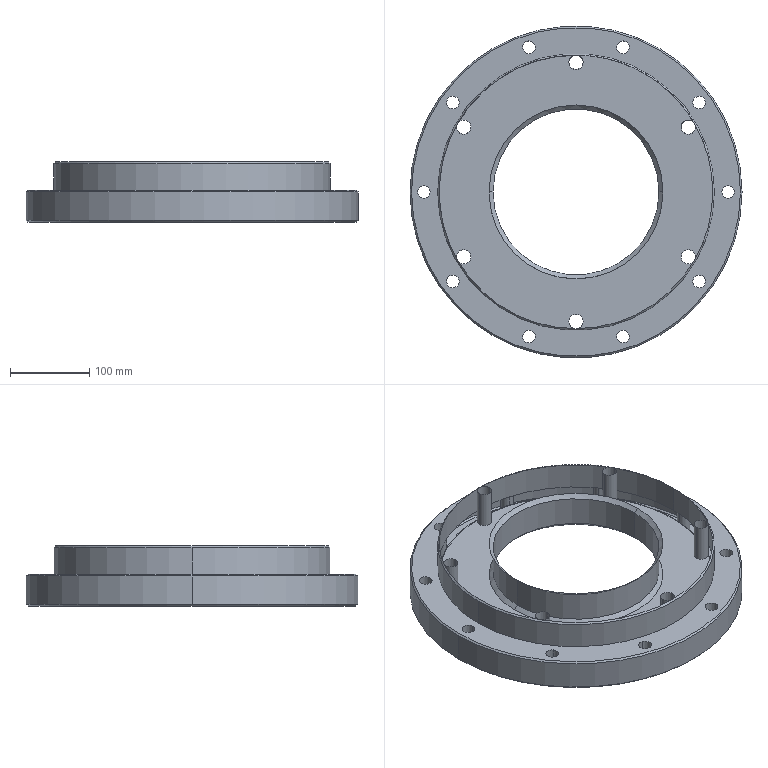Part | SolidWorks | features BaseBody 1 | 1 solid | 55 faces | box 420 x 420 x 76 mm | volume 4501710 mm3 | cylinder 40 | cone 10 | plane 5 | commonest cylinder face diameters 16 x20 18 x12 210 x2 348 x2 350 x2 420 x2